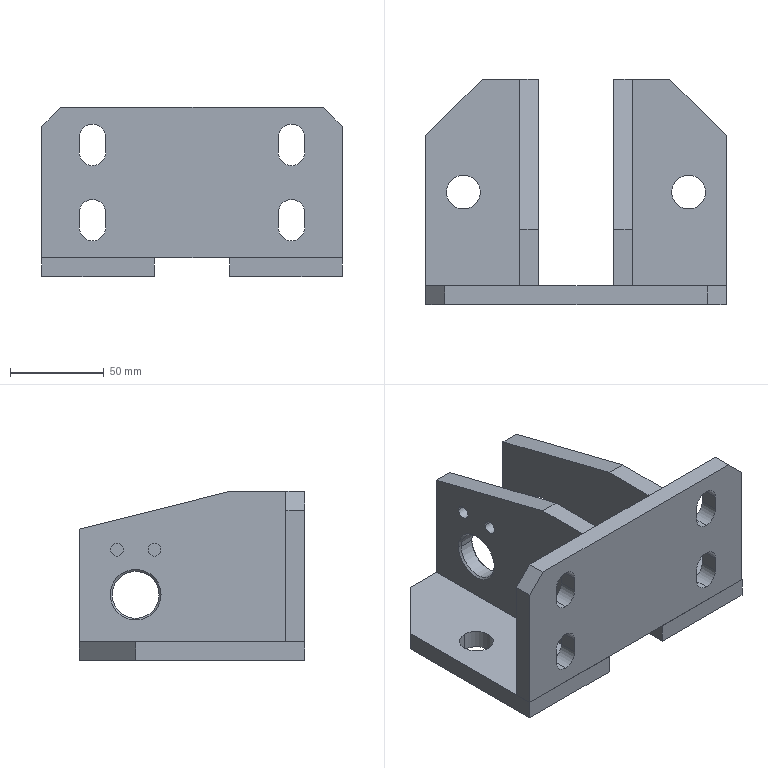Part | STEP file | 5 solids | 76 faces | box 160 x 120 x 90 mm | volume 395568 mm3 | plane 44 | cylinder 24 | cone 8 | commonest cylinder face diameters 14 x12 6.8 x4 18 x4 25 x4